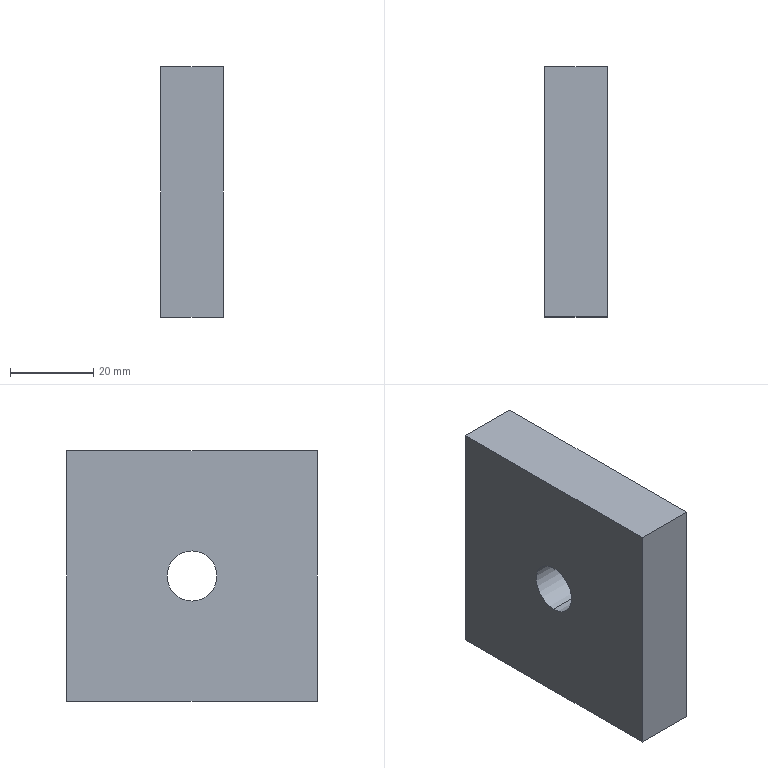Part | NX | 1 solid | 8 faces | box 15 x 60 x 60 mm | volume 52304 mm3 | plane 6 | cylinder 2 | commonest cylinder face diameters 12 x2
STEP:
#1=CARTESIAN_POINT('',(211.374,-541.499,2416.086));
#2=VERTEX_POINT('',#1);
#3=CARTESIAN_POINT('',(211.374,-541.499,2404.086));
#4=VERTEX_POINT('',#3);
#5=CARTESIAN_POINT('',(211.374,-541.499,2410.086));
#6=DIRECTION('',(1.,0.,0.));
#7=DIRECTION('',(0.,-1.,0.));
#8=AXIS2_PLACEMENT_3D('',#5,#6,#7);
#9=CIRCLE('',#8,6.);
#10=EDGE_CURVE('',#2,#4,#9,.T.);
#11=ORIENTED_EDGE('',*,*,#10,.F.);
#12=CARTESIAN_POINT('',(226.374,-541.499,2416.086));
#13=VERTEX_POINT('',#12);
#14=CARTESIAN_POINT('',(-4.626,-541.499,2416.086));
#15=DIRECTION('',(-1.,0.,0.));
#16=VECTOR('',#15,1.);
#17=LINE('',#14,#16);
#18=EDGE_CURVE('',#13,#2,#17,.T.);
#19=ORIENTED_EDGE('',*,*,#18,.F.);
#20=CARTESIAN_POINT('',(226.374,-541.499,2404.086));
#21=VERTEX_POINT('',#20);
#22=CARTESIAN_POINT('',(226.374,-541.499,2410.086));
#23=DIRECTION('',(1.,0.,0.));
#24=DIRECTION('',(0.,-1.,0.));
#25=AXIS2_PLACEMENT_3D('',#22,#23,#24);
#26=CIRCLE('',#25,6.);
#27=EDGE_CURVE('',#13,#21,#26,.T.);
#28=ORIENTED_EDGE('',*,*,#27,.T.);
#29=CARTESIAN_POINT('',(-4.626,-541.499,2404.086));
#30=DIRECTION('',(1.,0.,0.));
#31=VECTOR('',#30,1.);
#32=LINE('',#29,#31);
#33=EDGE_CURVE('',#4,#21,#32,.T.);
#34=ORIENTED_EDGE('',*,*,#33,.F.);
#35=EDGE_LOOP('',(#11,#19,#28,#34));
#36=FACE_OUTER_BOUND('',#35,.T.);
#37=CARTESIAN_POINT('',(-4.626,-541.499,2410.086));
#38=DIRECTION('',(1.,0.,0.));
#39=DIRECTION('',(0.,0.,-1.));
#40=AXIS2_PLACEMENT_3D('',#37,#38,#39);
#41=CYLINDRICAL_SURFACE('',#40,6.);
#42=ADVANCED_FACE('',(#36),#41,.F.);
#43=CARTESIAN_POINT('',(211.374,-511.499,2380.086));
#44=VERTEX_POINT('',#43);
#45=CARTESIAN_POINT('',(211.374,-571.499,2380.086));
#46=VERTEX_POINT('',#45);
#47=CARTESIAN_POINT('',(211.374,-511.499,2380.086));
#48=DIRECTION('',(0.,-1.,0.));
#49=VECTOR('',#48,1.);
#50=LINE('',#47,#49);
#51=EDGE_CURVE('',#44,#46,#50,.T.);
#52=ORIENTED_EDGE('',*,*,#51,.F.);
#53=CARTESIAN_POINT('',(226.374,-511.499,2380.086));
#54=VERTEX_POINT('',#53);
#55=CARTESIAN_POINT('',(226.374,-511.499,2380.086));
#56=DIRECTION('',(-1.,0.,0.));
#57=VECTOR('',#56,1.);
#58=LINE('',#55,#57);
#59=EDGE_CURVE('',#54,#44,#58,.T.);
#60=ORIENTED_EDGE('',*,*,#59,.F.);
#61=CARTESIAN_POINT('',(226.374,-571.499,2380.086));
#62=VERTEX_POINT('',#61);
#63=CARTESIAN_POINT('',(226.374,-511.499,2380.086));
#64=DIRECTION('',(0.,-1.,0.));
#65=VECTOR('',#64,1.);
#66=LINE('',#63,#65);
#67=EDGE_CURVE('',#54,#62,#66,.T.);
#68=ORIENTED_EDGE('',*,*,#67,.T.);
#69=CARTESIAN_POINT('',(226.374,-571.499,2380.086));
#70=DIRECTION('',(-1.,0.,0.));
#71=VECTOR('',#70,1.);
#72=LINE('',#69,#71);
#73=EDGE_CURVE('',#62,#46,#72,.T.);
#74=ORIENTED_EDGE('',*,*,#73,.T.);
#75=EDGE_LOOP('',(#52,#60,#68,#74));
#76=FACE_OUTER_BOUND('',#75,.T.);
#77=CARTESIAN_POINT('',(226.374,-511.499,2380.086));
#78=DIRECTION('',(0.,0.,1.));
#79=DIRECTION('',(0.,-1.,0.));
#80=AXIS2_PLACEMENT_3D('',#77,#78,#79);
#81=PLANE('',#80);
#82=ADVANCED_FACE('',(#76),#81,.F.);
#83=CARTESIAN_POINT('',(211.374,-571.499,2440.086));
#84=VERTEX_POINT('',#83);
#85=CARTESIAN_POINT('',(211.374,-571.499,2380.086));
#86=DIRECTION('',(0.,0.,1.));
#87=VECTOR('',#86,1.);
#88=LINE('',#85,#87);
#89=EDGE_CURVE('',#46,#84,#88,.T.);
#90=ORIENTED_EDGE('',*,*,#89,.F.);
#91=ORIENTED_EDGE('',*,*,#73,.F.);
#92=CARTESIAN_POINT('',(226.374,-571.499,2440.086));
#93=VERTEX_POINT('',#92);
#94=CARTESIAN_POINT('',(226.374,-571.499,2380.086));
#95=DIRECTION('',(0.,0.,1.));
#96=VECTOR('',#95,1.);
#97=LINE('',#94,#96);
#98=EDGE_CURVE('',#62,#93,#97,.T.);
#99=ORIENTED_EDGE('',*,*,#98,.T.);
#100=CARTESIAN_POINT('',(226.374,-571.499,2440.086));
#101=DIRECTION('',(-1.,0.,0.));
#102=VECTOR('',#101,1.);
#103=LINE('',#100,#102);
#104=EDGE_CURVE('',#93,#84,#103,.T.);
#105=ORIENTED_EDGE('',*,*,#104,.T.);
#106=EDGE_LOOP('',(#90,#91,#99,#105));
#107=FACE_OUTER_BOUND('',#106,.T.);
#108=CARTESIAN_POINT('',(226.374,-571.499,2380.086));
#109=DIRECTION('',(0.,1.,0.));
#110=DIRECTION('',(-1.,0.,0.));
#111=AXIS2_PLACEMENT_3D('',#108,#109,#110);
#112=PLANE('',#111);
#113=ADVANCED_FACE('',(#107),#112,.F.);
#114=CARTESIAN_POINT('',(211.374,-511.499,2440.086));
#115=VERTEX_POINT('',#114);
#116=CARTESIAN_POINT('',(211.374,-511.499,2440.086));
#117=DIRECTION('',(0.,1.,0.));
#118=VECTOR('',#117,1.);
#119=LINE('',#116,#118);
#120=EDGE_CURVE('',#84,#115,#119,.T.);
#121=ORIENTED_EDGE('',*,*,#120,.F.);
#122=ORIENTED_EDGE('',*,*,#104,.F.);
#123=CARTESIAN_POINT('',(226.374,-511.499,2440.086));
#124=VERTEX_POINT('',#123);
#125=CARTESIAN_POINT('',(226.374,-511.499,2440.086));
#126=DIRECTION('',(0.,1.,0.));
#127=VECTOR('',#126,1.);
#128=LINE('',#125,#127);
#129=EDGE_CURVE('',#93,#124,#128,.T.);
#130=ORIENTED_EDGE('',*,*,#129,.T.);
#131=CARTESIAN_POINT('',(226.374,-511.499,2440.086));
#132=DIRECTION('',(-1.,0.,0.));
#133=VECTOR('',#132,1.);
#134=LINE('',#131,#133);
#135=EDGE_CURVE('',#124,#115,#134,.T.);
#136=ORIENTED_EDGE('',*,*,#135,.T.);
#137=EDGE_LOOP('',(#121,#122,#130,#136));
#138=FACE_OUTER_BOUND('',#137,.T.);
#139=CARTESIAN_POINT('',(226.374,-511.499,2440.086));
#140=DIRECTION('',(0.,0.,-1.));
#141=DIRECTION('',(1.,0.,0.));
#142=AXIS2_PLACEMENT_3D('',#139,#140,#141);
#143=PLANE('',#142);
#144=ADVANCED_FACE('',(#138),#143,.F.);
#145=CARTESIAN_POINT('',(211.374,-511.499,2380.086));
#146=DIRECTION('',(0.,0.,-1.));
#147=VECTOR('',#146,1.);
#148=LINE('',#145,#147);
#149=EDGE_CURVE('',#115,#44,#148,.T.);
#150=ORIENTED_EDGE('',*,*,#149,.F.);
#151=ORIENTED_EDGE('',*,*,#135,.F.);
#152=CARTESIAN_POINT('',(226.374,-511.499,2380.086));
#153=DIRECTION('',(0.,0.,-1.));
#154=VECTOR('',#153,1.);
#155=LINE('',#152,#154);
#156=EDGE_CURVE('',#124,#54,#155,.T.);
#157=ORIENTED_EDGE('',*,*,#156,.T.);
#158=ORIENTED_EDGE('',*,*,#59,.T.);
#159=EDGE_LOOP('',(#150,#151,#157,#158));
#160=FACE_OUTER_BOUND('',#159,.T.);
#161=CARTESIAN_POINT('',(226.374,-511.499,2380.086));
#162=DIRECTION('',(0.,-1.,0.));
#163=DIRECTION('',(1.,0.,0.));
#164=AXIS2_PLACEMENT_3D('',#161,#162,#163);
#165=PLANE('',#164);
#166=ADVANCED_FACE('',(#160),#165,.F.);
#167=CARTESIAN_POINT('',(226.374,-541.499,2410.086));
#168=DIRECTION('',(1.,0.,0.));
#169=DIRECTION('',(0.,-1.,0.));
#170=AXIS2_PLACEMENT_3D('',#167,#168,#169);
#171=CIRCLE('',#170,6.);
#172=EDGE_CURVE('',#21,#13,#171,.T.);
#173=ORIENTED_EDGE('',*,*,#172,.F.);
#174=ORIENTED_EDGE('',*,*,#27,.F.);
#175=EDGE_LOOP('',(#173,#174));
#176=FACE_BOUND('',#175,.T.);
#177=ORIENTED_EDGE('',*,*,#67,.F.);
#178=ORIENTED_EDGE('',*,*,#156,.F.);
#179=ORIENTED_EDGE('',*,*,#129,.F.);
#180=ORIENTED_EDGE('',*,*,#98,.F.);
#181=EDGE_LOOP('',(#177,#178,#179,#180));
#182=FACE_BOUND('',#181,.T.);
#183=CARTESIAN_POINT('',(226.374,-571.499,2380.086));
#184=DIRECTION('',(1.,0.,0.));
#185=DIRECTION('',(0.,1.,0.));
#186=AXIS2_PLACEMENT_3D('',#183,#184,#185);
#187=PLANE('',#186);
#188=ADVANCED_FACE('',(#176,#182),#187,.T.);
#189=CARTESIAN_POINT('',(211.374,-541.499,2410.086));
#190=DIRECTION('',(1.,0.,0.));
#191=DIRECTION('',(0.,-1.,0.));
#192=AXIS2_PLACEMENT_3D('',#189,#190,#191);
#193=CIRCLE('',#192,6.);
#194=EDGE_CURVE('',#4,#2,#193,.T.);
#195=ORIENTED_EDGE('',*,*,#194,.T.);
#196=ORIENTED_EDGE('',*,*,#10,.T.);
#197=EDGE_LOOP('',(#195,#196));
#198=FACE_BOUND('',#197,.T.);
#199=ORIENTED_EDGE('',*,*,#51,.T.);
#200=ORIENTED_EDGE('',*,*,#89,.T.);
#201=ORIENTED_EDGE('',*,*,#120,.T.);
#202=ORIENTED_EDGE('',*,*,#149,.T.);
#203=EDGE_LOOP('',(#199,#200,#201,#202));
#204=FACE_BOUND('',#203,.T.);
#205=CARTESIAN_POINT('',(211.374,-571.499,2380.086));
#206=DIRECTION('',(1.,0.,0.));
#207=DIRECTION('',(0.,1.,0.));
#208=AXIS2_PLACEMENT_3D('',#205,#206,#207);
#209=PLANE('',#208);
#210=ADVANCED_FACE('',(#198,#204),#209,.F.);
#211=ORIENTED_EDGE('',*,*,#18,.T.);
#212=ORIENTED_EDGE('',*,*,#194,.F.);
#213=ORIENTED_EDGE('',*,*,#33,.T.);
#214=ORIENTED_EDGE('',*,*,#172,.T.);
#215=EDGE_LOOP('',(#211,#212,#213,#214));
#216=FACE_OUTER_BOUND('',#215,.T.);
#217=CARTESIAN_POINT('',(-4.626,-541.499,2410.086));
#218=DIRECTION('',(1.,0.,0.));
#219=DIRECTION('',(0.,0.,-1.));
#220=AXIS2_PLACEMENT_3D('',#217,#218,#219);
#221=CYLINDRICAL_SURFACE('',#220,6.);
#222=ADVANCED_FACE('',(#216),#221,.F.);
#223=CLOSED_SHELL('',(#42,#82,#113,#144,#166,#188,#210,#222));
#224=MANIFOLD_SOLID_BREP('',#223);
#225=(LENGTH_UNIT()NAMED_UNIT(*)SI_UNIT(.MILLI.,.METRE.));
#226=UNCERTAINTY_MEASURE_WITH_UNIT(LENGTH_MEASURE(0.00002),#225,'','');
#227=(NAMED_UNIT(*)PLANE_ANGLE_UNIT()SI_UNIT($,.RADIAN.));
#228=PLANE_ANGLE_MEASURE_WITH_UNIT(PLANE_ANGLE_MEASURE(0.01745),#227);
#229=DIMENSIONAL_EXPONENTS(0.,0.,0.,0.,0.,0.,0.);
#230=(CONVERSION_BASED_UNIT('DEGREE',#228)NAMED_UNIT(#229)PLANE_ANGLE_UNIT());
#231=(NAMED_UNIT(*)SI_UNIT($,.STERADIAN.)SOLID_ANGLE_UNIT());
#232=(GEOMETRIC_REPRESENTATION_CONTEXT(3)GLOBAL_UNCERTAINTY_ASSIGNED_CONTEXT((#226))GLOBAL_UNIT_ASSIGNED_CONTEXT((#225,#230,#231))REPRESENTATION_CONTEXT('',''));
#233=ADVANCED_BREP_SHAPE_REPRESENTATION('',(#224),#232);